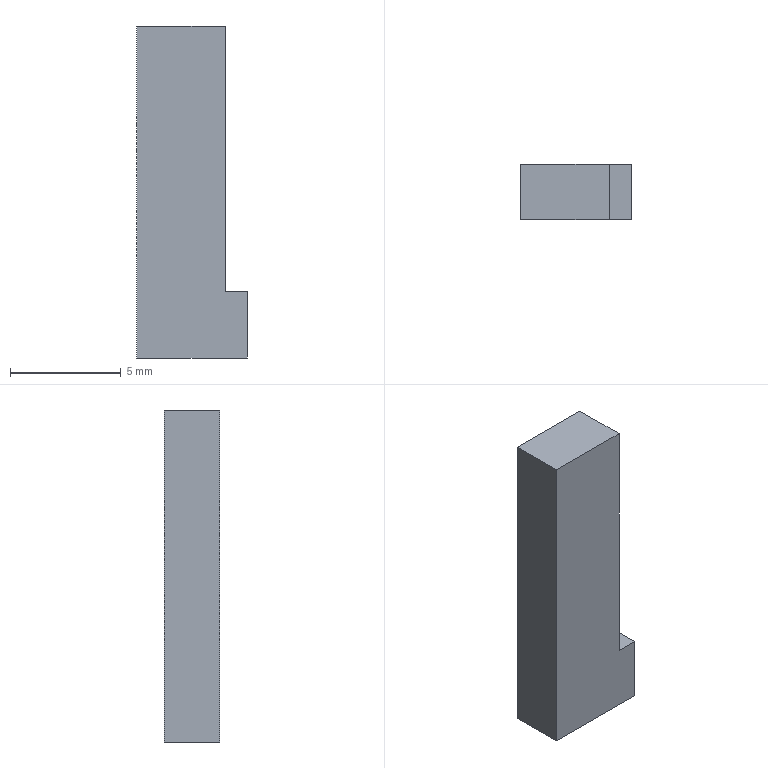Part | NX | features DIE-25 2 | 1 solid | 8 faces | box 5 x 2.5 x 15 mm | volume 157.5 mm3 | plane 8
STEP:
#1=CARTESIAN_POINT('',(2449.31,-843.773,846.716));
#2=VERTEX_POINT('',#1);
#3=CARTESIAN_POINT('',(2449.31,-846.273,846.716));
#4=VERTEX_POINT('',#3);
#5=CARTESIAN_POINT('',(2449.31,-844.398,846.716));
#6=DIRECTION('',(0.,1.,0.));
#7=VECTOR('',#6,1000.);
#8=LINE('',#5,#7);
#9=EDGE_CURVE('',#2,#4,#8,.F.);
#10=ORIENTED_EDGE('',*,*,#9,.F.);
#11=CARTESIAN_POINT('',(2449.31,-843.773,858.716));
#12=VERTEX_POINT('',#11);
#13=CARTESIAN_POINT('',(2449.31,-843.773,858.516));
#14=DIRECTION('',(0.,0.,-1.));
#15=VECTOR('',#14,1000.);
#16=LINE('',#13,#15);
#17=EDGE_CURVE('',#2,#12,#16,.F.);
#18=ORIENTED_EDGE('',*,*,#17,.T.);
#19=CARTESIAN_POINT('',(2449.31,-846.273,858.716));
#20=VERTEX_POINT('',#19);
#21=CARTESIAN_POINT('',(2449.31,-845.023,858.716));
#22=DIRECTION('',(0.,-1.,0.));
#23=VECTOR('',#22,1000.);
#24=LINE('',#21,#23);
#25=EDGE_CURVE('',#12,#20,#24,.T.);
#26=ORIENTED_EDGE('',*,*,#25,.T.);
#27=CARTESIAN_POINT('',(2449.31,-846.273,858.516));
#28=DIRECTION('',(0.,0.,-1.));
#29=VECTOR('',#28,1000.);
#30=LINE('',#27,#29);
#31=EDGE_CURVE('',#4,#20,#30,.F.);
#32=ORIENTED_EDGE('',*,*,#31,.F.);
#33=EDGE_LOOP('',(#10,#18,#26,#32));
#34=FACE_BOUND('',#33,.T.);
#35=CARTESIAN_POINT('',(2449.31,-844.398,858.516));
#36=DIRECTION('',(-1.,0.,0.));
#37=DIRECTION('',(0.,0.,1.));
#38=AXIS2_PLACEMENT_3D('',#35,#36,#37);
#39=PLANE('',#38);
#40=ADVANCED_FACE('',(#34),#39,.F.);
#41=ORIENTED_EDGE('',*,*,#25,.F.);
#42=CARTESIAN_POINT('',(2445.31,-843.773,858.716));
#43=VERTEX_POINT('',#42);
#44=CARTESIAN_POINT('',(2447.31,-843.773,858.716));
#45=DIRECTION('',(1.,0.,0.));
#46=VECTOR('',#45,1000.);
#47=LINE('',#44,#46);
#48=EDGE_CURVE('',#12,#43,#47,.F.);
#49=ORIENTED_EDGE('',*,*,#48,.T.);
#50=CARTESIAN_POINT('',(2445.31,-846.273,858.716));
#51=VERTEX_POINT('',#50);
#52=CARTESIAN_POINT('',(2445.31,-845.023,858.716));
#53=DIRECTION('',(0.,-1.,0.));
#54=VECTOR('',#53,1000.);
#55=LINE('',#52,#54);
#56=EDGE_CURVE('',#43,#51,#55,.T.);
#57=ORIENTED_EDGE('',*,*,#56,.T.);
#58=CARTESIAN_POINT('',(2447.31,-846.273,858.716));
#59=DIRECTION('',(1.,0.,0.));
#60=VECTOR('',#59,1000.);
#61=LINE('',#58,#60);
#62=EDGE_CURVE('',#20,#51,#61,.F.);
#63=ORIENTED_EDGE('',*,*,#62,.F.);
#64=EDGE_LOOP('',(#41,#49,#57,#63));
#65=FACE_BOUND('',#64,.T.);
#66=CARTESIAN_POINT('',(2447.31,-845.023,858.716));
#67=DIRECTION('',(0.,0.,1.));
#68=DIRECTION('',(1.,0.,0.));
#69=AXIS2_PLACEMENT_3D('',#66,#67,#68);
#70=PLANE('',#69);
#71=ADVANCED_FACE('',(#65),#70,.T.);
#72=CARTESIAN_POINT('',(2445.31,-843.773,843.716));
#73=VERTEX_POINT('',#72);
#74=CARTESIAN_POINT('',(2445.31,-843.773,858.516));
#75=DIRECTION('',(0.,0.,-1.));
#76=VECTOR('',#75,1000.);
#77=LINE('',#74,#76);
#78=EDGE_CURVE('',#73,#43,#77,.F.);
#79=ORIENTED_EDGE('',*,*,#78,.F.);
#80=CARTESIAN_POINT('',(2445.31,-846.273,843.716));
#81=VERTEX_POINT('',#80);
#82=CARTESIAN_POINT('',(2445.31,-844.398,843.716));
#83=DIRECTION('',(0.,-1.,0.));
#84=VECTOR('',#83,1000.);
#85=LINE('',#82,#84);
#86=EDGE_CURVE('',#73,#81,#85,.T.);
#87=ORIENTED_EDGE('',*,*,#86,.T.);
#88=CARTESIAN_POINT('',(2445.31,-846.273,858.516));
#89=DIRECTION('',(0.,0.,-1.));
#90=VECTOR('',#89,1000.);
#91=LINE('',#88,#90);
#92=EDGE_CURVE('',#81,#51,#91,.F.);
#93=ORIENTED_EDGE('',*,*,#92,.T.);
#94=ORIENTED_EDGE('',*,*,#56,.F.);
#95=EDGE_LOOP('',(#79,#87,#93,#94));
#96=FACE_BOUND('',#95,.T.);
#97=CARTESIAN_POINT('',(2445.31,-844.398,858.516));
#98=DIRECTION('',(1.,0.,0.));
#99=DIRECTION('',(0.,0.,1.));
#100=AXIS2_PLACEMENT_3D('',#97,#98,#99);
#101=PLANE('',#100);
#102=ADVANCED_FACE('',(#96),#101,.F.);
#103=ORIENTED_EDGE('',*,*,#92,.F.);
#104=CARTESIAN_POINT('',(2450.31,-846.273,843.716));
#105=VERTEX_POINT('',#104);
#106=CARTESIAN_POINT('',(2448.697,-846.273,843.716));
#107=DIRECTION('',(1.,0.,0.));
#108=VECTOR('',#107,1000.);
#109=LINE('',#106,#108);
#110=EDGE_CURVE('',#81,#105,#109,.T.);
#111=ORIENTED_EDGE('',*,*,#110,.T.);
#112=CARTESIAN_POINT('',(2450.31,-846.273,846.716));
#113=VERTEX_POINT('',#112);
#114=CARTESIAN_POINT('',(2450.31,-846.273,858.516));
#115=DIRECTION('',(0.,0.,-1.));
#116=VECTOR('',#115,1000.);
#117=LINE('',#114,#116);
#118=EDGE_CURVE('',#105,#113,#117,.F.);
#119=ORIENTED_EDGE('',*,*,#118,.T.);
#120=CARTESIAN_POINT('',(2449.31,-846.273,846.716));
#121=DIRECTION('',(1.,0.,0.));
#122=VECTOR('',#121,1000.);
#123=LINE('',#120,#122);
#124=EDGE_CURVE('',#113,#4,#123,.F.);
#125=ORIENTED_EDGE('',*,*,#124,.T.);
#126=ORIENTED_EDGE('',*,*,#31,.T.);
#127=ORIENTED_EDGE('',*,*,#62,.T.);
#128=EDGE_LOOP('',(#103,#111,#119,#125,#126,#127));
#129=FACE_BOUND('',#128,.T.);
#130=CARTESIAN_POINT('',(2448.697,-846.273,858.516));
#131=DIRECTION('',(0.,1.,0.));
#132=DIRECTION('',(0.,0.,-1.));
#133=AXIS2_PLACEMENT_3D('',#130,#131,#132);
#134=PLANE('',#133);
#135=ADVANCED_FACE('',(#129),#134,.F.);
#136=ORIENTED_EDGE('',*,*,#17,.F.);
#137=CARTESIAN_POINT('',(2450.31,-843.773,846.716));
#138=VERTEX_POINT('',#137);
#139=CARTESIAN_POINT('',(2449.31,-843.773,846.716));
#140=DIRECTION('',(1.,0.,0.));
#141=VECTOR('',#140,1000.);
#142=LINE('',#139,#141);
#143=EDGE_CURVE('',#138,#2,#142,.F.);
#144=ORIENTED_EDGE('',*,*,#143,.F.);
#145=CARTESIAN_POINT('',(2450.31,-843.773,843.716));
#146=VERTEX_POINT('',#145);
#147=CARTESIAN_POINT('',(2450.31,-843.773,858.516));
#148=DIRECTION('',(0.,0.,-1.));
#149=VECTOR('',#148,1000.);
#150=LINE('',#147,#149);
#151=EDGE_CURVE('',#146,#138,#150,.F.);
#152=ORIENTED_EDGE('',*,*,#151,.F.);
#153=CARTESIAN_POINT('',(2448.697,-843.773,843.716));
#154=DIRECTION('',(-1.,0.,0.));
#155=VECTOR('',#154,1000.);
#156=LINE('',#153,#155);
#157=EDGE_CURVE('',#146,#73,#156,.T.);
#158=ORIENTED_EDGE('',*,*,#157,.T.);
#159=ORIENTED_EDGE('',*,*,#78,.T.);
#160=ORIENTED_EDGE('',*,*,#48,.F.);
#161=EDGE_LOOP('',(#136,#144,#152,#158,#159,#160));
#162=FACE_BOUND('',#161,.T.);
#163=CARTESIAN_POINT('',(2448.697,-843.773,858.516));
#164=DIRECTION('',(0.,-1.,0.));
#165=DIRECTION('',(0.,0.,-1.));
#166=AXIS2_PLACEMENT_3D('',#163,#164,#165);
#167=PLANE('',#166);
#168=ADVANCED_FACE('',(#162),#167,.F.);
#169=ORIENTED_EDGE('',*,*,#157,.F.);
#170=CARTESIAN_POINT('',(2450.31,-844.398,843.716));
#171=DIRECTION('',(0.,1.,0.));
#172=VECTOR('',#171,1000.);
#173=LINE('',#170,#172);
#174=EDGE_CURVE('',#146,#105,#173,.F.);
#175=ORIENTED_EDGE('',*,*,#174,.T.);
#176=ORIENTED_EDGE('',*,*,#110,.F.);
#177=ORIENTED_EDGE('',*,*,#86,.F.);
#178=EDGE_LOOP('',(#169,#175,#176,#177));
#179=FACE_BOUND('',#178,.T.);
#180=CARTESIAN_POINT('',(2447.31,-845.023,843.716));
#181=DIRECTION('',(0.,0.,1.));
#182=DIRECTION('',(1.,0.,0.));
#183=AXIS2_PLACEMENT_3D('',#180,#181,#182);
#184=PLANE('',#183);
#185=ADVANCED_FACE('',(#179),#184,.F.);
#186=ORIENTED_EDGE('',*,*,#9,.T.);
#187=ORIENTED_EDGE('',*,*,#124,.F.);
#188=CARTESIAN_POINT('',(2450.31,-844.398,846.716));
#189=DIRECTION('',(0.,1.,0.));
#190=VECTOR('',#189,1000.);
#191=LINE('',#188,#190);
#192=EDGE_CURVE('',#113,#138,#191,.T.);
#193=ORIENTED_EDGE('',*,*,#192,.T.);
#194=ORIENTED_EDGE('',*,*,#143,.T.);
#195=EDGE_LOOP('',(#186,#187,#193,#194));
#196=FACE_BOUND('',#195,.T.);
#197=CARTESIAN_POINT('',(2449.81,-845.023,846.716));
#198=DIRECTION('',(0.,0.,1.));
#199=DIRECTION('',(1.,0.,0.));
#200=AXIS2_PLACEMENT_3D('',#197,#198,#199);
#201=PLANE('',#200);
#202=ADVANCED_FACE('',(#196),#201,.T.);
#203=ORIENTED_EDGE('',*,*,#192,.F.);
#204=ORIENTED_EDGE('',*,*,#118,.F.);
#205=ORIENTED_EDGE('',*,*,#174,.F.);
#206=ORIENTED_EDGE('',*,*,#151,.T.);
#207=EDGE_LOOP('',(#203,#204,#205,#206));
#208=FACE_BOUND('',#207,.T.);
#209=CARTESIAN_POINT('',(2450.31,-844.398,858.516));
#210=DIRECTION('',(-1.,0.,0.));
#211=DIRECTION('',(0.,0.,1.));
#212=AXIS2_PLACEMENT_3D('',#209,#210,#211);
#213=PLANE('',#212);
#214=ADVANCED_FACE('',(#208),#213,.F.);
#215=CLOSED_SHELL('',(#40,#71,#102,#135,#168,#185,#202,#214));
#216=MANIFOLD_SOLID_BREP('',#215);
#217=(LENGTH_UNIT()NAMED_UNIT(*)SI_UNIT(.MILLI.,.METRE.));
#218=UNCERTAINTY_MEASURE_WITH_UNIT(LENGTH_MEASURE(0.00001),#217,'','');
#219=(NAMED_UNIT(*)PLANE_ANGLE_UNIT()SI_UNIT($,.RADIAN.));
#220=(NAMED_UNIT(*)SI_UNIT($,.STERADIAN.)SOLID_ANGLE_UNIT());
#221=(GEOMETRIC_REPRESENTATION_CONTEXT(3)GLOBAL_UNCERTAINTY_ASSIGNED_CONTEXT((#218))GLOBAL_UNIT_ASSIGNED_CONTEXT((#217,#219,#220))REPRESENTATION_CONTEXT('',''));
#222=ADVANCED_BREP_SHAPE_REPRESENTATION('',(#216),#221);